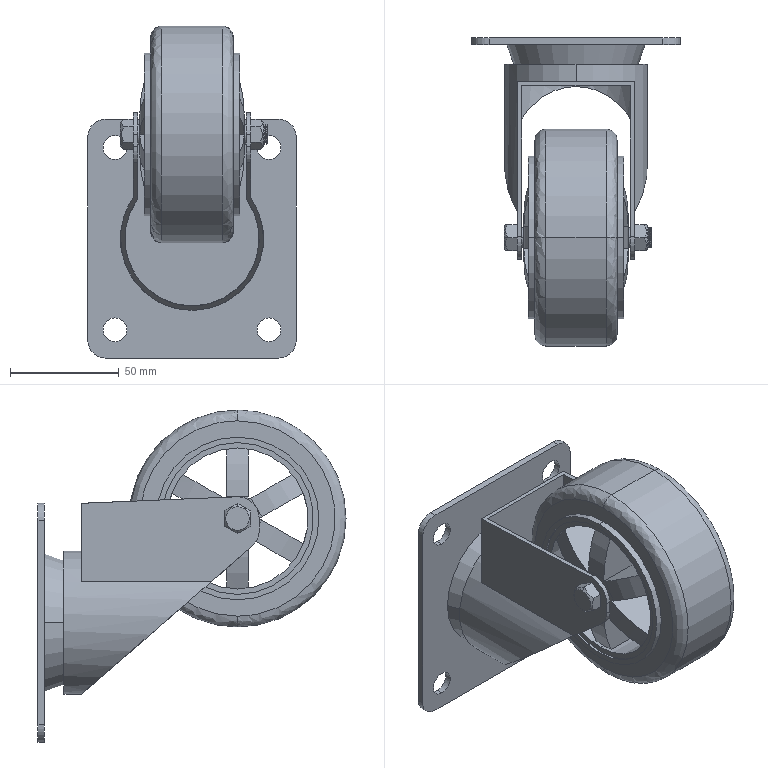Part | SolidWorks | features BaseBody 1 | 1 solid | 125 faces | box 96 x 142 x 153 mm | volume 354889 mm3 | plane 55 | cylinder 54 | spline 8 | cone 8 | commonest cylinder face diameters 106.25 x12 9 x9 11 x8 16 x4 20 x4 70 x4